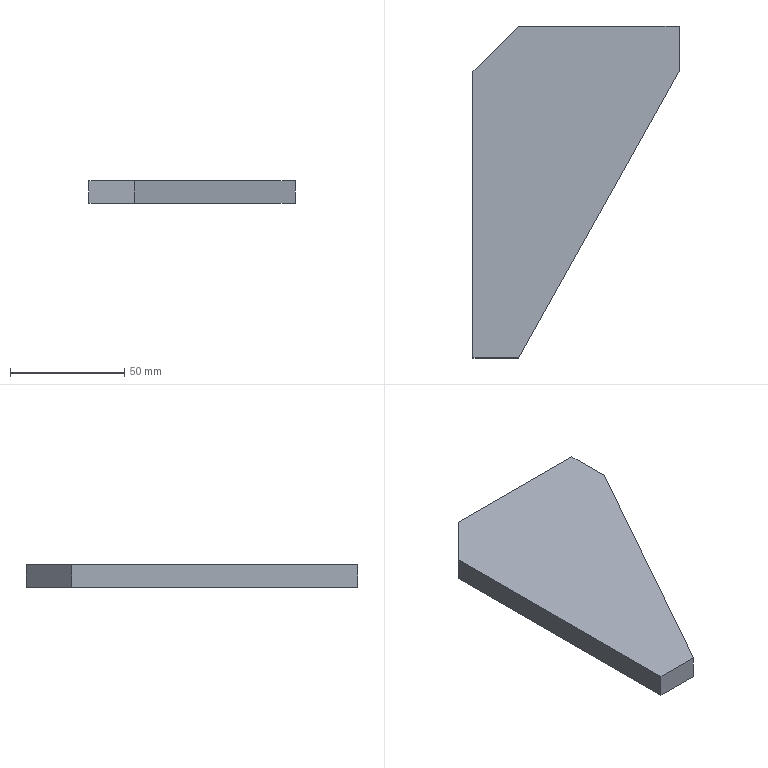Part | SolidWorks | features Extrusion 1 | 1 solid | 8 faces | box 90 x 145 x 10 mm | volume 84750 mm3 | plane 8
STEP:
#1=CARTESIAN_POINT('',(0.,125.,0.));
#2=VERTEX_POINT('',#1);
#3=CARTESIAN_POINT('',(0.,0.,0.));
#4=VERTEX_POINT('',#3);
#5=CARTESIAN_POINT('',(0.,125.,0.));
#6=DIRECTION('',(0.,-1.,0.));
#7=VECTOR('',#6,1000.);
#8=LINE('',#5,#7);
#9=EDGE_CURVE('',#2,#4,#8,.T.);
#10=ORIENTED_EDGE('',*,*,#9,.T.);
#11=CARTESIAN_POINT('',(0.,0.,10.));
#12=VERTEX_POINT('',#11);
#13=CARTESIAN_POINT('',(0.,0.,10.));
#14=DIRECTION('',(0.,0.,-1.));
#15=VECTOR('',#14,1000.);
#16=LINE('',#13,#15);
#17=EDGE_CURVE('',#12,#4,#16,.T.);
#18=ORIENTED_EDGE('',*,*,#17,.F.);
#19=CARTESIAN_POINT('',(0.,125.,10.));
#20=VERTEX_POINT('',#19);
#21=CARTESIAN_POINT('',(0.,125.,10.));
#22=DIRECTION('',(0.,-1.,0.));
#23=VECTOR('',#22,1000.);
#24=LINE('',#21,#23);
#25=EDGE_CURVE('',#20,#12,#24,.T.);
#26=ORIENTED_EDGE('',*,*,#25,.F.);
#27=CARTESIAN_POINT('',(0.,125.,10.));
#28=DIRECTION('',(0.,0.,-1.));
#29=VECTOR('',#28,1000.);
#30=LINE('',#27,#29);
#31=EDGE_CURVE('',#20,#2,#30,.T.);
#32=ORIENTED_EDGE('',*,*,#31,.T.);
#33=EDGE_LOOP('',(#10,#18,#26,#32));
#34=FACE_OUTER_BOUND('',#33,.T.);
#35=CARTESIAN_POINT('',(0.,125.,10.));
#36=DIRECTION('',(1.,0.,0.));
#37=DIRECTION('',(0.,1.,0.));
#38=AXIS2_PLACEMENT_3D('',#35,#36,#37);
#39=PLANE('',#38);
#40=ADVANCED_FACE('',(#34),#39,.F.);
#41=CARTESIAN_POINT('',(20.,0.,0.));
#42=VERTEX_POINT('',#41);
#43=CARTESIAN_POINT('',(0.,0.,0.));
#44=DIRECTION('',(1.,0.,0.));
#45=VECTOR('',#44,1000.);
#46=LINE('',#43,#45);
#47=EDGE_CURVE('',#4,#42,#46,.T.);
#48=ORIENTED_EDGE('',*,*,#47,.T.);
#49=CARTESIAN_POINT('',(20.,0.,10.));
#50=VERTEX_POINT('',#49);
#51=CARTESIAN_POINT('',(20.,0.,10.));
#52=DIRECTION('',(0.,0.,-1.));
#53=VECTOR('',#52,1000.);
#54=LINE('',#51,#53);
#55=EDGE_CURVE('',#50,#42,#54,.T.);
#56=ORIENTED_EDGE('',*,*,#55,.F.);
#57=CARTESIAN_POINT('',(0.,0.,10.));
#58=DIRECTION('',(1.,0.,0.));
#59=VECTOR('',#58,1000.);
#60=LINE('',#57,#59);
#61=EDGE_CURVE('',#12,#50,#60,.T.);
#62=ORIENTED_EDGE('',*,*,#61,.F.);
#63=ORIENTED_EDGE('',*,*,#17,.T.);
#64=EDGE_LOOP('',(#48,#56,#62,#63));
#65=FACE_OUTER_BOUND('',#64,.T.);
#66=CARTESIAN_POINT('',(0.,0.,10.));
#67=DIRECTION('',(0.,1.,0.));
#68=DIRECTION('',(0.,0.,1.));
#69=AXIS2_PLACEMENT_3D('',#66,#67,#68);
#70=PLANE('',#69);
#71=ADVANCED_FACE('',(#65),#70,.F.);
#72=CARTESIAN_POINT('',(90.,125.,0.));
#73=VERTEX_POINT('',#72);
#74=CARTESIAN_POINT('',(20.,0.,0.));
#75=DIRECTION('',(0.4886,0.8725,0.));
#76=VECTOR('',#75,1000.);
#77=LINE('',#74,#76);
#78=EDGE_CURVE('',#42,#73,#77,.T.);
#79=ORIENTED_EDGE('',*,*,#78,.T.);
#80=CARTESIAN_POINT('',(90.,125.,10.));
#81=VERTEX_POINT('',#80);
#82=CARTESIAN_POINT('',(90.,125.,10.));
#83=DIRECTION('',(0.,0.,-1.));
#84=VECTOR('',#83,1000.);
#85=LINE('',#82,#84);
#86=EDGE_CURVE('',#81,#73,#85,.T.);
#87=ORIENTED_EDGE('',*,*,#86,.F.);
#88=CARTESIAN_POINT('',(20.,0.,10.));
#89=DIRECTION('',(0.4886,0.8725,0.));
#90=VECTOR('',#89,1000.);
#91=LINE('',#88,#90);
#92=EDGE_CURVE('',#50,#81,#91,.T.);
#93=ORIENTED_EDGE('',*,*,#92,.F.);
#94=ORIENTED_EDGE('',*,*,#55,.T.);
#95=EDGE_LOOP('',(#79,#87,#93,#94));
#96=FACE_OUTER_BOUND('',#95,.T.);
#97=CARTESIAN_POINT('',(20.,0.,10.));
#98=DIRECTION('',(-0.8725,0.4886,0.));
#99=DIRECTION('',(-0.4886,-0.8725,0.));
#100=AXIS2_PLACEMENT_3D('',#97,#98,#99);
#101=PLANE('',#100);
#102=ADVANCED_FACE('',(#96),#101,.F.);
#103=CARTESIAN_POINT('',(90.,145.,0.));
#104=VERTEX_POINT('',#103);
#105=CARTESIAN_POINT('',(90.,125.,0.));
#106=DIRECTION('',(0.,1.,0.));
#107=VECTOR('',#106,1000.);
#108=LINE('',#105,#107);
#109=EDGE_CURVE('',#73,#104,#108,.T.);
#110=ORIENTED_EDGE('',*,*,#109,.T.);
#111=CARTESIAN_POINT('',(90.,145.,10.));
#112=VERTEX_POINT('',#111);
#113=CARTESIAN_POINT('',(90.,145.,10.));
#114=DIRECTION('',(0.,0.,-1.));
#115=VECTOR('',#114,1000.);
#116=LINE('',#113,#115);
#117=EDGE_CURVE('',#112,#104,#116,.T.);
#118=ORIENTED_EDGE('',*,*,#117,.F.);
#119=CARTESIAN_POINT('',(90.,125.,10.));
#120=DIRECTION('',(0.,1.,0.));
#121=VECTOR('',#120,1000.);
#122=LINE('',#119,#121);
#123=EDGE_CURVE('',#81,#112,#122,.T.);
#124=ORIENTED_EDGE('',*,*,#123,.F.);
#125=ORIENTED_EDGE('',*,*,#86,.T.);
#126=EDGE_LOOP('',(#110,#118,#124,#125));
#127=FACE_OUTER_BOUND('',#126,.T.);
#128=CARTESIAN_POINT('',(90.,125.,10.));
#129=DIRECTION('',(-1.,0.,0.));
#130=DIRECTION('',(0.,0.,1.));
#131=AXIS2_PLACEMENT_3D('',#128,#129,#130);
#132=PLANE('',#131);
#133=ADVANCED_FACE('',(#127),#132,.F.);
#134=CARTESIAN_POINT('',(20.,145.,0.));
#135=VERTEX_POINT('',#134);
#136=CARTESIAN_POINT('',(90.,145.,0.));
#137=DIRECTION('',(-1.,0.,0.));
#138=VECTOR('',#137,1000.);
#139=LINE('',#136,#138);
#140=EDGE_CURVE('',#104,#135,#139,.T.);
#141=ORIENTED_EDGE('',*,*,#140,.T.);
#142=CARTESIAN_POINT('',(20.,145.,10.));
#143=VERTEX_POINT('',#142);
#144=CARTESIAN_POINT('',(20.,145.,10.));
#145=DIRECTION('',(0.,0.,-1.));
#146=VECTOR('',#145,1000.);
#147=LINE('',#144,#146);
#148=EDGE_CURVE('',#143,#135,#147,.T.);
#149=ORIENTED_EDGE('',*,*,#148,.F.);
#150=CARTESIAN_POINT('',(90.,145.,10.));
#151=DIRECTION('',(-1.,0.,0.));
#152=VECTOR('',#151,1000.);
#153=LINE('',#150,#152);
#154=EDGE_CURVE('',#112,#143,#153,.T.);
#155=ORIENTED_EDGE('',*,*,#154,.F.);
#156=ORIENTED_EDGE('',*,*,#117,.T.);
#157=EDGE_LOOP('',(#141,#149,#155,#156));
#158=FACE_OUTER_BOUND('',#157,.T.);
#159=CARTESIAN_POINT('',(90.,145.,10.));
#160=DIRECTION('',(0.,-1.,0.));
#161=DIRECTION('',(0.,0.,-1.));
#162=AXIS2_PLACEMENT_3D('',#159,#160,#161);
#163=PLANE('',#162);
#164=ADVANCED_FACE('',(#158),#163,.F.);
#165=CARTESIAN_POINT('',(20.,145.,0.));
#166=DIRECTION('',(-0.7071,-0.7071,0.));
#167=VECTOR('',#166,1000.);
#168=LINE('',#165,#167);
#169=EDGE_CURVE('',#135,#2,#168,.T.);
#170=ORIENTED_EDGE('',*,*,#169,.T.);
#171=ORIENTED_EDGE('',*,*,#31,.F.);
#172=CARTESIAN_POINT('',(20.,145.,10.));
#173=DIRECTION('',(-0.7071,-0.7071,0.));
#174=VECTOR('',#173,1000.);
#175=LINE('',#172,#174);
#176=EDGE_CURVE('',#143,#20,#175,.T.);
#177=ORIENTED_EDGE('',*,*,#176,.F.);
#178=ORIENTED_EDGE('',*,*,#148,.T.);
#179=EDGE_LOOP('',(#170,#171,#177,#178));
#180=FACE_OUTER_BOUND('',#179,.T.);
#181=CARTESIAN_POINT('',(20.,145.,10.));
#182=DIRECTION('',(0.7071,-0.7071,0.));
#183=DIRECTION('',(0.7071,0.7071,0.));
#184=AXIS2_PLACEMENT_3D('',#181,#182,#183);
#185=PLANE('',#184);
#186=ADVANCED_FACE('',(#180),#185,.F.);
#187=ORIENTED_EDGE('',*,*,#25,.T.);
#188=ORIENTED_EDGE('',*,*,#61,.T.);
#189=ORIENTED_EDGE('',*,*,#92,.T.);
#190=ORIENTED_EDGE('',*,*,#123,.T.);
#191=ORIENTED_EDGE('',*,*,#154,.T.);
#192=ORIENTED_EDGE('',*,*,#176,.T.);
#193=EDGE_LOOP('',(#187,#188,#189,#190,#191,#192));
#194=FACE_OUTER_BOUND('',#193,.T.);
#195=CARTESIAN_POINT('',(0.,0.,10.));
#196=DIRECTION('',(0.,0.,1.));
#197=DIRECTION('',(1.,0.,0.));
#198=AXIS2_PLACEMENT_3D('',#195,#196,#197);
#199=PLANE('',#198);
#200=ADVANCED_FACE('',(#194),#199,.T.);
#201=ORIENTED_EDGE('',*,*,#9,.F.);
#202=ORIENTED_EDGE('',*,*,#169,.F.);
#203=ORIENTED_EDGE('',*,*,#140,.F.);
#204=ORIENTED_EDGE('',*,*,#109,.F.);
#205=ORIENTED_EDGE('',*,*,#78,.F.);
#206=ORIENTED_EDGE('',*,*,#47,.F.);
#207=EDGE_LOOP('',(#201,#202,#203,#204,#205,#206));
#208=FACE_OUTER_BOUND('',#207,.T.);
#209=CARTESIAN_POINT('',(0.,0.,0.));
#210=DIRECTION('',(0.,0.,1.));
#211=DIRECTION('',(1.,0.,0.));
#212=AXIS2_PLACEMENT_3D('',#209,#210,#211);
#213=PLANE('',#212);
#214=ADVANCED_FACE('',(#208),#213,.F.);
#215=CLOSED_SHELL('',(#40,#71,#102,#133,#164,#186,#200,#214));
#216=MANIFOLD_SOLID_BREP('',#215);
#217=CARTESIAN_POINT('',(0.,0.,0.));
#218=DIRECTION('',(0.,0.,1.));
#219=DIRECTION('',(1.,0.,0.));
#220=AXIS2_PLACEMENT_3D('',#217,#218,#219);
#221=(LENGTH_UNIT()NAMED_UNIT(*)SI_UNIT(.MILLI.,.METRE.));
#222=UNCERTAINTY_MEASURE_WITH_UNIT(LENGTH_MEASURE(0.00001),#221,'','');
#223=(NAMED_UNIT(*)PLANE_ANGLE_UNIT()SI_UNIT($,.RADIAN.));
#224=(NAMED_UNIT(*)SI_UNIT($,.STERADIAN.)SOLID_ANGLE_UNIT());
#225=(GEOMETRIC_REPRESENTATION_CONTEXT(3)GLOBAL_UNCERTAINTY_ASSIGNED_CONTEXT((#222))GLOBAL_UNIT_ASSIGNED_CONTEXT((#221,#223,#224))REPRESENTATION_CONTEXT('',''));
#226=ADVANCED_BREP_SHAPE_REPRESENTATION('',(#216,#220),#225);